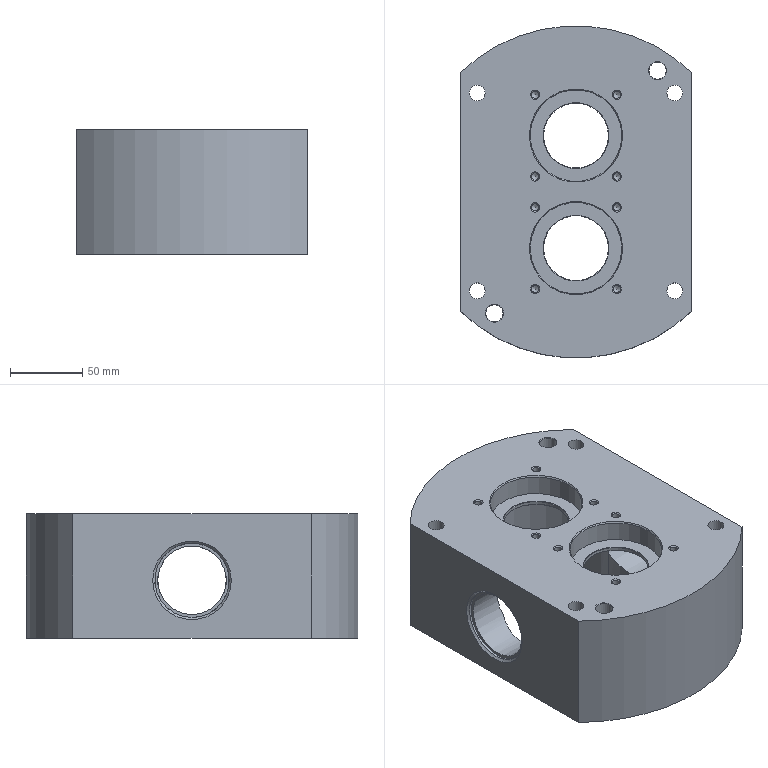NC program | NX | posted with a generic post | part box 160 x 230 x 86 mm
Lines 1 to 2290 of 2342, first 2014 of 2276 lines:
N10 G17 G21 G94 G90
(FLOOR_WALL , TOOL : D50)
N12 T02 M6
N14 G54
N16 G17 G0 G90 X46.956 Y-52.997 B0. C0. S1200 M3
N18 G43 Z30. H2
N20 Z2.651
N22 G94 G1 Z-0.349 F1000.
N24 X43.956
N26 X-43.956 F2000.
N28 Y-24.331
N30 X43.956
N32 Y4.334
N34 X-43.956
N36 Y33.
N38 X43.956
N40 X46.956
N42 Z2.651
N44 G0 Z30.
N46 X50.654 Y-52.997
N48 Z2.302
N50 G1 Z-0.698 F1000.
N52 X47.654
N54 X-47.654 F2000.
N56 Y-24.331
N58 X47.654
N60 Y4.334
N62 X-47.654
N64 Y33.
N66 X47.654
N68 X50.654
N70 Z2.302
N72 G0 Z30.
N74 X53.485 Y-52.997
N76 Z1.953
N78 G1 Z-1.047 F1000.
N80 X50.485
N82 X-50.485 F2000.
N84 Y-24.331
N86 X50.485
N88 Y4.334
N90 X-50.485
N92 Y33.
N94 X50.485
N96 X53.485
N98 Z1.953
N100 G0 Z30.
N102 X55.866 Y-52.997
N104 Z1.604
N106 G1 Z-1.396 F1000.
N108 X52.866
N110 X-52.866 F2000.
N112 Y-24.331
N114 X52.866
N116 Y4.334
N118 X-52.866
N120 Y33.
N122 X52.866
N124 X55.866
N126 Z1.604
N128 G0 Z30.
N130 X57.959 Y-52.997
N132 Z1.255
N134 G1 Z-1.745 F1000.
N136 X54.959
N138 X-54.959 F2000.
N140 Y-24.331
N142 X54.959
N144 Y4.334
N146 X-54.959
N148 Y33.
N150 X54.959
N152 X57.959
N154 Z1.255
N156 G0 Z30.
N158 X59.847 Y-52.997
N160 Z0.906
N162 G1 Z-2.094 F1000.
N164 X56.847
N166 X-56.847 F2000.
N168 Y-24.331
N170 X56.847
N172 Y4.334
N174 X-56.847
N176 Y33.
N178 X56.847
N180 X59.847
N182 Z0.906
N184 G0 Z30.
N186 X61.579 Y-52.997
N188 Z0.557
N190 G1 Z-2.443 F1000.
N192 X58.579
N194 X-58.579 F2000.
N196 Y-24.331
N198 X58.579
N200 Y4.334
N202 X-58.579
N204 Y33.
N206 X58.579
N208 X61.579
N210 Z0.557
N212 G0 Z30.
N214 X63.188 Y-52.997
N216 Z0.208
N218 G1 Z-2.792 F1000.
N220 X60.188
N222 X-60.188 F2000.
N224 Y-24.331
N226 X60.188
N228 Y4.334
N230 X-60.188
N232 Y33.
N234 X60.188
N236 X63.188
N238 Z0.208
N240 G0 Z30.
N242 X64.695 Y-52.997
N244 Z-0.141
N246 G1 Z-3.141 F1000.
N248 X61.695
N250 X-61.695 F2000.
N252 Y-24.331
N254 X61.695
N256 Y4.334
N258 X-61.695
N260 Y33.
N262 X61.695
N264 X64.695
N266 Z-0.141
N268 G0 Z30.
N270 X66.117 Y-52.997
N272 Z-0.49
N274 G1 Z-3.49 F1000.
N276 X63.117
N278 X-63.117 F2000.
N280 Y-24.331
N282 X63.117
N284 Y4.334
N286 X-63.117
N288 Y33.
N290 X63.117
N292 X66.117
N294 Z-0.49
N296 G0 Z30.
N298 X67.467 Y-52.997
N300 Z-0.839
N302 G1 Z-3.839 F1000.
N304 X64.467
N306 X-64.467 F2000.
N308 Y-24.331
N310 X64.467
N312 Y4.334
N314 X-64.467
N316 Y33.
N318 X64.467
N320 X67.467
N322 Z-0.839
N324 G0 Z30.
N326 X68.753 Y-52.997
N328 Z-1.188
N330 G1 Z-4.188 F1000.
N332 X65.753
N334 X-65.753 F2000.
N336 Y-24.331
N338 X65.753
N340 Y4.334
N342 X-65.753
N344 Y33.
N346 X65.753
N348 X68.753
N350 Z-1.188
N352 G0 Z30.
N354 X69.984 Y-52.997
N356 Z-1.537
N358 G1 Z-4.537 F1000.
N360 X66.984
N362 X-66.984 F2000.
N364 Y-24.331
N366 X66.984
N368 Y4.334
N370 X-66.984
N372 Y33.
N374 X66.984
N376 X69.984
N378 Z-1.537
N380 G0 Z30.
N382 X71.166 Y-52.997
N384 Z-1.886
N386 G1 Z-4.886 F1000.
N388 X68.166
N390 X-68.166 F2000.
N392 Y-24.331
N394 X68.166
N396 Y4.334
N398 X-68.166
N400 Y33.
N402 X68.166
N404 X71.166
N406 Z-1.886
N408 G0 Z30.
N410 X72.303 Y-52.997
N412 Z-2.235
N414 G1 Z-5.235 F1000.
N416 X69.303
N418 X-69.303 F2000.
N420 Y-24.331
N422 X69.303
N424 Y4.334
N426 X-69.303
N428 Y33.
N430 X69.303
N432 X72.303
N434 Z-2.235
N436 G0 Z30.
N438 X73.4 Y-52.997
N440 Z-2.584
N442 G1 Z-5.584 F1000.
N444 X70.4
N446 X-70.4 F2000.
N448 Y-24.331
N450 X70.4
N452 Y4.334
N454 X-70.4
N456 Y33.
N458 X70.4
N460 X73.4
N462 Z-2.584
N464 G0 Z30.
N466 X74.462 Y-52.997
N468 Z-2.933
N470 G1 Z-5.933 F1000.
N472 X71.462
N474 X-71.462 F2000.
N476 Y-24.331
N478 X71.462
N480 Y4.334
N482 X-71.462
N484 Y33.
N486 X71.462
N488 X74.462
N490 Z-2.933
N492 G0 Z30.
N494 X75.489 Y-52.997
N496 Z-3.282
N498 G1 Z-6.282 F1000.
N500 X72.489
N502 X-72.489 F2000.
N504 Y-24.331
N506 X72.489
N508 Y4.334
N510 X-72.489
N512 Y33.
N514 X72.489
N516 X75.489
N518 Z-3.282
N520 G0 Z30.
N522 X76.487 Y-52.997
N524 Z-3.631
N526 G1 Z-6.631 F1000.
N528 X73.487
N530 X-73.487 F2000.
N532 Y-24.331
N534 X73.487
N536 Y4.334
N538 X-73.487
N540 Y33.
N542 X73.487
N544 X76.487
N546 Z-3.631
N548 G0 Z30.
N550 X77.455 Y-52.997
N552 Z-3.98
N554 G1 Z-6.98 F1000.
N556 X74.455
N558 X-74.455 F2000.
N560 Y-24.331
N562 X74.455
N564 Y4.334
N566 X-74.455
N568 Y33.
N570 X74.455
N572 X77.455
N574 Z-3.98
N576 G0 Z30.
N578 X78.398 Y-52.997
N580 Z-4.329
N582 G1 Z-7.329 F1000.
N584 X75.398
N586 X-75.398 F2000.
N588 Y-24.331
N590 X75.398
N592 Y4.334
N594 X-75.398
N596 Y33.
N598 X75.398
N600 X78.398
N602 Z-4.329
N604 G0 Z30.
N606 X79.316 Y-52.997
N608 Z-4.678
N610 G1 Z-7.678 F1000.
N612 X76.316
N614 X-76.316 F2000.
N616 Y-24.331
N618 X76.316
N620 Y4.334
N622 X-76.316
N624 Y33.
N626 X76.316
N628 X79.316
N630 Z-4.678
N632 G0 Z30.
N634 X80.212 Y-52.997
N636 Z-5.027
N638 G1 Z-8.027 F1000.
N640 X77.212
N642 X-77.212 F2000.
N644 Y-24.331
N646 X77.212
N648 Y4.334
N650 X-77.212
N652 Y33.
N654 X77.212
N656 X80.212
N658 Z-5.027
N660 G0 Z30.
N662 X81.086 Y-52.997
N664 Z-5.376
N666 G1 Z-8.376 F1000.
N668 X78.086
N670 X-78.086 F2000.
N672 Y-24.331
N674 X78.086
N676 Y4.334
N678 X-78.086
N680 Y33.
N682 X78.086
N684 X81.086
N686 Z-5.376
N688 G0 Z30.
N690 X81.939 Y-52.997
N692 Z-5.725
N694 G1 Z-8.725 F1000.
N696 X78.939
N698 X-78.939 F2000.
N700 Y-24.331
N702 X78.939
N704 Y4.334
N706 X-78.939
N708 Y33.
N710 X78.939
N712 X81.939
N714 Z-5.725
N716 G0 Z30.
N718 X82.774 Y-52.997
N720 Z-6.074
N722 G1 Z-9.074 F1000.
N724 X79.774
N726 X-79.774 F2000.
N728 Y-24.331
N730 X79.774
N732 Y4.334
N734 X-79.774
N736 Y33.
N738 X79.774
N740 X82.774
N742 Z-6.074
N744 G0 Z30.
N746 X83.591 Y-52.997
N748 Z-6.423
N750 G1 Z-9.423 F1000.
N752 X80.591
N754 X-80.591 F2000.
N756 Y-24.331
N758 X80.591
N760 Y4.334
N762 X-80.591
N764 Y33.
N766 X80.591
N768 X83.591
N770 Z-6.423
N772 G0 Z30.
N774 X84.391 Y-52.997
N776 Z-6.772
N778 G1 Z-9.772 F1000.
N780 X81.391
N782 X-81.391 F2000.
N784 Y-24.331
N786 X81.391
N788 Y4.334
N790 X-81.391
N792 Y33.
N794 X81.391
N796 X84.391
N798 Z-6.772
N800 G0 Z30.
N802 X85.175 Y-52.997
N804 Z-7.121
N806 G1 Z-10.121 F1000.
N808 X82.175
N810 X-82.175 F2000.
N812 Y-24.331
N814 X82.175
N816 Y4.334
N818 X-82.175
N820 Y33.
N822 X82.175
N824 X85.175
N826 Z-7.121
N828 G0 Z30.
N830 X85.943 Y-52.997
N832 Z-7.47
N834 G1 Z-10.47 F1000.
N836 X82.943
N838 X-82.943 F2000.
N840 Y-24.331
N842 X82.943
N844 Y4.334
N846 X-82.943
N848 Y33.
N850 X82.943
N852 X85.943
N854 Z-7.47
N856 G0 Z30.
N858 X86.697 Y-52.997
N860 Z-7.819
N862 G1 Z-10.819 F1000.
N864 X83.697
N866 X-83.697 F2000.
N868 Y-24.331
N870 X83.697
N872 Y4.334
N874 X-83.697
N876 Y33.
N878 X83.697
N880 X86.697
N882 Z-7.819
N884 G0 Z30.
N886 X87.436 Y-52.997
N888 Z-8.168
N890 G1 Z-11.168 F1000.
N892 X84.436
N894 X-84.436 F2000.
N896 Y-24.331
N898 X84.436
N900 Y4.334
N902 X-84.436
N904 Y33.
N906 X84.436
N908 X87.436
N910 Z-8.168
N912 G0 Z30.
N914 X88.163 Y-52.997
N916 Z-8.517
N918 G1 Z-11.517 F1000.
N920 X85.163
N922 X-85.163 F2000.
N924 Y-24.331
N926 X85.163
N928 Y4.334
N930 X-85.163
N932 Y33.
N934 X85.163
N936 X88.163
N938 Z-8.517
N940 G0 Z30.
N942 X88.877 Y-52.997
N944 Z-8.866
N946 G1 Z-11.866 F1000.
N948 X85.877
N950 X-85.877 F2000.
N952 Y-24.331
N954 X85.877
N956 Y4.334
N958 X-85.877
N960 Y33.
N962 X85.877
N964 X88.877
N966 Z-8.866
N968 G0 Z30.
N970 X89.578 Y-52.997
N972 Z-9.215
N974 G1 Z-12.215 F1000.
N976 X86.578
N978 X-86.578 F2000.
N980 Y-24.331
N982 X86.578
N984 Y4.334
N986 X-86.578
N988 Y33.
N990 X86.578
N992 X89.578
N994 Z-9.215
N996 G0 Z30.
N998 X90.268 Y-52.997
N1000 Z-9.564
N1002 G1 Z-12.564 F1000.
N1004 X87.268
N1006 X-87.268 F2000.
N1008 Y-24.331
N1010 X87.268
N1012 Y4.334
N1014 X-87.268
N1016 Y33.
N1018 X87.268
N1020 X90.268
N1022 Z-9.564
N1024 G0 Z30.
N1026 X90.946 Y-52.997
N1028 Z-9.913
N1030 G1 Z-12.913 F1000.
N1032 X87.946
N1034 X-87.946 F2000.
N1036 Y-24.331
N1038 X87.946
N1040 Y4.334
N1042 X-87.946
N1044 Y33.
N1046 X87.946
N1048 X90.946
N1050 Z-9.913
N1052 G0 Z30.
N1054 X91.614 Y-52.997
N1056 Z-10.262
N1058 G1 Z-13.262 F1000.
N1060 X88.614
N1062 X-88.614 F2000.
N1064 Y-24.331
N1066 X88.614
N1068 Y4.334
N1070 X-88.614
N1072 Y33.
N1074 X88.614
N1076 X91.614
N1078 Z-10.262
N1080 G0 Z30.
N1082 X92.271 Y-52.997
N1084 Z-10.611
N1086 G1 Z-13.611 F1000.
N1088 X89.271
N1090 X-89.271 F2000.
N1092 Y-24.331
N1094 X89.271
N1096 Y4.334
N1098 X-89.271
N1100 Y33.
N1102 X89.271
N1104 X92.271
N1106 Z-10.611
N1108 G0 Z30.
N1110 X92.918 Y-52.997
N1112 Z-10.96
N1114 G1 Z-13.96 F1000.
N1116 X89.918
N1118 X-89.918 F2000.
N1120 Y-24.331
N1122 X89.918
N1124 Y4.334
N1126 X-89.918
N1128 Y33.
N1130 X89.918
N1132 X92.918
N1134 Z-10.96
N1136 G0 Z30.
N1138 X93.555 Y-52.997
N1140 Z-11.309
N1142 G1 Z-14.309 F1000.
N1144 X90.555
N1146 X-90.555 F2000.
N1148 Y-24.331
N1150 X90.555
N1152 Y4.334
N1154 X-90.555
N1156 Y33.
N1158 X90.555
N1160 X93.555
N1162 Z-11.309
N1164 G0 Z30.
N1166 X94.183 Y-52.997
N1168 Z-11.658
N1170 G1 Z-14.658 F1000.
N1172 X91.183
N1174 X-91.183 F2000.
N1176 Y-24.331
N1178 X91.183
N1180 Y4.334
N1182 X-91.183
N1184 Y33.
N1186 X91.183
N1188 X94.183
N1190 Z-11.658
N1192 G0 Z30.
N1194 X94.802 Y-52.997
N1196 Z-12.007
N1198 G1 Z-15.007 F1000.
N1200 X91.802
N1202 X-91.802 F2000.
N1204 Y-24.331
N1206 X91.802
N1208 Y4.334
N1210 X-91.802
N1212 Y33.
N1214 X91.802
N1216 X94.802
N1218 Z-12.007
N1220 G0 Z30.
N1222 X95.412 Y-52.997
N1224 Z-12.356
N1226 G1 Z-15.356 F1000.
N1228 X92.412
N1230 X-92.412 F2000.
N1232 Y-24.331
N1234 X92.412
N1236 Y4.334
N1238 X-92.412
N1240 Y33.
N1242 X92.412
N1244 X95.412
N1246 Z-12.356
N1248 G0 Z30.
N1250 X96.013 Y-52.997
N1252 Z-12.705
N1254 G1 Z-15.705 F1000.
N1256 X93.013
N1258 X-93.013 F2000.
N1260 Y-24.331
N1262 X93.013
N1264 Y4.334
N1266 X-93.013
N1268 Y33.
N1270 X93.013
N1272 X96.013
N1274 Z-12.705
N1276 G0 Z30.
N1278 X96.606 Y-52.997
N1280 Z-13.054
N1282 G1 Z-16.054 F1000.
N1284 X93.606
N1286 X-93.606 F2000.
N1288 Y-24.331
N1290 X93.606
N1292 Y4.334
N1294 X-93.606
N1296 Y33.
N1298 X93.606
N1300 X96.606
N1302 Z-13.054
N1304 G0 Z30.
N1306 X97.192 Y-52.997
N1308 Z-13.403
N1310 G1 Z-16.403 F1000.
N1312 X94.192
N1314 X-94.192 F2000.
N1316 Y-24.331
N1318 X94.192
N1320 Y4.334
N1322 X-94.192
N1324 Y33.
N1326 X94.192
N1328 X97.192
N1330 Z-13.403
N1332 G0 Z30.
N1334 X97.769 Y-52.997
N1336 Z-13.752
N1338 G1 Z-16.752 F1000.
N1340 X94.769
N1342 X-94.769 F2000.
N1344 Y-24.331
N1346 X94.769
N1348 Y4.334
N1350 X-94.769
N1352 Y33.
N1354 X94.769
N1356 X97.769
N1358 Z-13.752
N1360 G0 Z30.
N1362 X98.339 Y-52.997
N1364 Z-14.101
N1366 G1 Z-17.101 F1000.
N1368 X95.339
N1370 X-95.339 F2000.
N1372 Y-24.331
N1374 X95.339
N1376 Y4.334
N1378 X-95.339
N1380 Y33.
N1382 X95.339
N1384 X98.339
N1386 Z-14.101
N1388 G0 Z30.
N1390 X98.902 Y-52.997
N1392 Z-14.45
N1394 G1 Z-17.45 F1000.
N1396 X95.902
N1398 X-95.902 F2000.
N1400 Y-24.331
N1402 X95.902
N1404 Y4.334
N1406 X-95.902
N1408 Y33.
N1410 X95.902
N1412 X98.902
N1414 Z-14.45
N1416 G0 Z30.
N1418 X99.457 Y-52.997
N1420 Z-14.799
N1422 G1 Z-17.799 F1000.
N1424 X96.457
N1426 X-96.457 F2000.
N1428 Y-24.331
N1430 X96.457
N1432 Y4.334
N1434 X-96.457
N1436 Y33.
N1438 X96.457
N1440 X99.457
N1442 Z-14.799
N1444 G0 Z30.
N1446 X100.006 Y-52.997
N1448 Z-15.148
N1450 G1 Z-18.148 F1000.
N1452 X97.006
N1454 X-97.006 F2000.
N1456 Y-24.331
N1458 X97.006
N1460 Y4.334
N1462 X-97.006
N1464 Y33.
N1466 X97.006
N1468 X100.006
N1470 Z-15.148
N1472 G0 Z30.
N1474 X100.548 Y-52.997
N1476 Z-15.497
N1478 G1 Z-18.497 F1000.
N1480 X97.548
N1482 X-97.548 F2000.
N1484 Y-24.331
N1486 X97.548
N1488 Y4.334
N1490 X-97.548
N1492 Y33.
N1494 X97.548
N1496 X100.548
N1498 Z-15.497
N1500 G0 Z30.
N1502 X101.083 Y-52.997
N1504 Z-15.846
N1506 G1 Z-18.846 F1000.
N1508 X98.083
N1510 X-98.083 F2000.
N1512 Y-24.331
N1514 X98.083
N1516 Y4.334
N1518 X-98.083
N1520 Y33.
N1522 X98.083
N1524 X101.083
N1526 Z-15.846
N1528 G0 Z30.
N1530 X101.612 Y-52.997
N1532 Z-16.195
N1534 G1 Z-19.195 F1000.
N1536 X98.612
N1538 X-98.612 F2000.
N1540 Y-24.331
N1542 X98.612
N1544 Y4.334
N1546 X-98.612
N1548 Y33.
N1550 X98.612
N1552 X101.612
N1554 Z-16.195
N1556 G0 Z30.
N1558 X102.134 Y-52.997
N1560 Z-16.544
N1562 G1 Z-19.544 F1000.
N1564 X99.134
N1566 X-99.134 F2000.
N1568 Y-24.331
N1570 X99.134
N1572 Y4.334
N1574 X-99.134
N1576 Y33.
N1578 X99.134
N1580 X102.134
N1582 Z-16.544
N1584 G0 Z30.
N1586 X102.65 Y-52.997
N1588 Z-16.893
N1590 G1 Z-19.893 F1000.
N1592 X99.65
N1594 X-99.65 F2000.
N1596 Y-24.331
N1598 X99.65
N1600 Y4.334
N1602 X-99.65
N1604 Y33.
N1606 X99.65
N1608 X102.65
N1610 Z-16.893
N1612 G0 Z30.
N1614 X103.161 Y-52.997
N1616 Z-17.242
N1618 G1 Z-20.242 F1000.
N1620 X100.161
N1622 X-100.161 F2000.
N1624 Y-24.331
N1626 X100.161
N1628 Y4.334
N1630 X-100.161
N1632 Y33.
N1634 X100.161
N1636 X103.161
N1638 Z-17.242
N1640 G0 Z30.
N1642 X103.666 Y-52.997
N1644 Z-17.591
N1646 G1 Z-20.591 F1000.
N1648 X100.666
N1650 X-100.666 F2000.
N1652 Y-24.331
N1654 X100.666
N1656 Y4.334
N1658 X-100.666
N1660 Y33.
N1662 X100.666
N1664 X103.666
N1666 Z-17.591
N1668 G0 Z30.
N1670 X104.164 Y-52.997
N1672 Z-17.94
N1674 G1 Z-20.94 F1000.
N1676 X101.164
N1678 X-101.164 F2000.
N1680 Y-24.331
N1682 X101.164
N1684 Y4.334
N1686 X-101.164
N1688 Y33.
N1690 X101.164
N1692 X104.164
N1694 Z-17.94
N1696 G0 Z30.
N1698 X104.658 Y-52.997
N1700 Z-18.289
N1702 G1 Z-21.289 F1000.
N1704 X101.658
N1706 X-101.658 F2000.
N1708 Y-24.331
N1710 X101.658
N1712 Y4.334
N1714 X-101.658
N1716 Y33.
N1718 X101.658
N1720 X104.658
N1722 Z-18.289
N1724 G0 Z30.
N1726 X105.146 Y-52.997
N1728 Z-18.638
N1730 G1 Z-21.638 F1000.
N1732 X102.146
N1734 X-102.146 F2000.
N1736 Y-24.331
N1738 X102.146
N1740 Y4.334
N1742 X-102.146
N1744 Y33.
N1746 X102.146
N1748 X105.146
N1750 Z-18.638
N1752 G0 Z30.
N1754 X105.628 Y-52.997
N1756 Z-18.987
N1758 G1 Z-21.987 F1000.
N1760 X102.628
N1762 X-102.628 F2000.
N1764 Y-24.331
N1766 X102.628
N1768 Y4.334
N1770 X-102.628
N1772 Y33.
N1774 X102.628
N1776 X105.628
N1778 Z-18.987
N1780 G0 Z30.
N1782 X106.106 Y-52.997
N1784 Z-19.336
N1786 G1 Z-22.336 F1000.
N1788 X103.106
N1790 X-103.106 F2000.
N1792 Y-24.331
N1794 X103.106
N1796 Y4.334
N1798 X-103.106
N1800 Y33.
N1802 X103.106
N1804 X106.106
N1806 Z-19.336
N1808 G0 Z30.
N1810 X106.578 Y-52.997
N1812 Z-19.685
N1814 G1 Z-22.685 F1000.
N1816 X103.578
N1818 X-103.578 F2000.
N1820 Y-24.331
N1822 X103.578
N1824 Y4.334
N1826 X-103.578
N1828 Y33.
N1830 X103.578
N1832 X106.578
N1834 Z-19.685
N1836 G0 Z30.
N1838 X107.045 Y-52.997
N1840 Z-20.034
N1842 G1 Z-23.034 F1000.
N1844 X104.045
N1846 X-104.045 F2000.
N1848 Y-24.331
N1850 X104.045
N1852 Y4.334
N1854 X-104.045
N1856 Y33.
N1858 X104.045
N1860 X107.045
N1862 Z-20.034
N1864 G0 Z30.
N1866 X107.508 Y-52.997
N1868 Z-20.383
N1870 G1 Z-23.383 F1000.
N1872 X104.508
N1874 X-104.508 F2000.
N1876 Y-24.331
N1878 X104.508
N1880 Y4.334
N1882 X-104.508
N1884 Y33.
N1886 X104.508
N1888 X107.508
N1890 Z-20.383
N1892 G0 Z30.
N1894 X107.965 Y-52.997
N1896 Z-20.732
N1898 G1 Z-23.732 F1000.
N1900 X104.965
N1902 X-104.965 F2000.
N1904 Y-24.331
N1906 X104.965
N1908 Y4.334
N1910 X-104.965
N1912 Y33.
N1914 X104.965
N1916 X107.965
N1918 Z-20.732
N1920 G0 Z30.
N1922 X108.418 Y-52.997
N1924 Z-21.081
N1926 G1 Z-24.081 F1000.
N1928 X105.418
N1930 X-105.418 F2000.
N1932 Y-24.331
N1934 X105.418
N1936 Y4.334
N1938 X-105.418
N1940 Y33.
N1942 X105.418
N1944 X108.418
N1946 Z-21.081
N1948 G0 Z30.
N1950 X108.867 Y-52.997
N1952 Z-21.43
N1954 G1 Z-24.43 F1000.
N1956 X105.867
N1958 X-105.867 F2000.
N1960 Y-24.331
N1962 X105.867
N1964 Y4.334
N1966 X-105.867
N1968 Y33.
N1970 X105.867
N1972 X108.867
N1974 Z-21.43
N1976 G0 Z30.
N1978 X109.31 Y-52.997
N1980 Z-21.779
N1982 G1 Z-24.779 F1000.
N1984 X106.31
N1986 X-106.31 F2000.
N1988 Y-24.331
N1990 X106.31
N1992 Y4.334
N1994 X-106.31
N1996 Y33.
N1998 X106.31
N2000 X109.31
N2002 Z-21.779
N2004 G0 Z30.
N2006 X109.75 Y-52.997
N2008 Z-22.128
N2010 G1 Z-25.128 F1000.
N2012 X106.75
N2014 X-106.75 F2000.
N2016 Y-24.331
N2018 X106.75
N2020 Y4.334
N2022 X-106.75
N2024 Y33.
N2026 X106.75
N2028 X109.75
N2030 Z-22.128
N2032 G0 Z30.
N2034 X110.185 Y-52.997
N2036 Z-22.477
N2038 G1 Z-25.477 F1000.
N2040 X107.185
N2042 X-107.185 F2000.
N2044 Y-24.331
N2046 X107.185
N2048 Y4.334
N2050 X-107.185
N2052 Y33.
N2054 X107.185
N2056 X110.185
N2058 Z-22.477
N2060 G0 Z30.
N2062 X110.616 Y-52.997
N2064 Z-22.826
N2066 G1 Z-25.826 F1000.
N2068 X107.616
N2070 X-107.616 F2000.
N2072 Y-24.331
N2074 X107.616
N2076 Y4.334
N2078 X-107.616
N2080 Y33.
N2082 X107.616
N2084 X110.616
N2086 Z-22.826
N2088 G0 Z30.
N2090 X111.042 Y-52.997
N2092 Z-23.175
N2094 G1 Z-26.175 F1000.
N2096 X108.042
N2098 X-108.042 F2000.
N2100 Y-24.331
N2102 X108.042
N2104 Y4.334
N2106 X-108.042
N2108 Y33.
N2110 X108.042
N2112 X111.042
N2114 Z-23.175
N2116 G0 Z30.
N2118 X111.464 Y-52.997
N2120 Z-23.524
N2122 G1 Z-26.524 F1000.
N2124 X108.464
N2126 X-108.464 F2000.
N2128 Y-24.331
N2130 X108.464
N2132 Y4.334
N2134 X-108.464
N2136 Y33.
N2138 X108.464
N2140 X111.464
N2142 Z-23.524
N2144 G0 Z30.
N2146 X111.883 Y-52.997
N2148 Z-23.873
N2150 G1 Z-26.873 F1000.
N2152 X108.883
N2154 X-108.883 F2000.
N2156 Y-24.331
N2158 X108.883
N2160 Y4.334
N2162 X-108.883
N2164 Y33.
N2166 X108.883
N2168 X111.883
N2170 Z-23.873
N2172 G0 Z30.
N2174 X112.297 Y-52.997
N2176 Z-24.222
N2178 G1 Z-27.222 F1000.
N2180 X109.297
N2182 X-109.297 F2000.
N2184 Y-24.331
N2186 X109.297
N2188 Y4.334
N2190 X-109.297
N2192 Y33.
N2194 X109.297
N2196 X112.297
N2198 Z-24.222
N2200 G0 Z30.
N2202 X112.707 Y-52.997
N2204 Z-24.571
N2206 G1 Z-27.571 F1000.
N2208 X109.707
N2210 X-109.707 F2000.
N2212 Y-24.331
N2214 X109.707
N2216 Y4.334
N2218 X-109.707
N2220 Y33.
N2222 X109.707
N2224 X112.707
N2226 Z-24.571
N2228 G0 Z30.
N2230 X113.114 Y-52.997
N2232 Z-24.92
N2234 G1 Z-27.92 F1000.
N2236 X110.114
N2238 X-110.114 F2000.
N2240 Y-24.331
N2242 X110.114
N2244 Y4.334
N2246 X-110.114
N2248 Y33.
N2250 X110.114
N2252 X113.114
N2254 Z-24.92
N2256 G0 Z30.
N2258 X113.517 Y-52.997
N2260 Z-25.269
N2262 G1 Z-28.269 F1000.
N2264 X110.517
N2266 X-110.517 F2000.
N2268 Y-24.331
N2270 X110.517
N2272 Y4.334
N2274 X-110.517
N2276 Y33.
N2278 X110.517
N2280 X113.517
N2282 Z-25.269
N2284 G0 Z30.
N2286 X113.915 Y-52.997
N2288 Z-25.618
N2290 G1 Z-28.618 F1000.
N2292 X110.915
N2294 X-110.915 F2000.
N2296 Y-24.331
N2298 X110.915
N2300 Y4.334
N2302 X-110.915
N2304 Y33.
N2306 X110.915
N2308 X113.915
N2310 Z-25.618
N2312 G0 Z30.
N2314 X114.311 Y-52.997
N2316 Z-25.967
N2318 G1 Z-28.967 F1000.
N2320 X111.311
N2322 X-111.311 F2000.
N2324 Y-24.331
N2326 X111.311
N2328 Y4.334
N2330 X-111.311
N2332 Y33.
N2334 X111.311
N2336 X114.311
N2338 Z-25.967
N2340 G0 Z30.
N2342 X114.702 Y-52.997
N2344 Z-26.316
N2346 G1 Z-29.316 F1000.
N2348 X111.702
N2350 X-111.702 F2000.
N2352 Y-24.331
N2354 X111.702
N2356 Y4.334
N2358 X-111.702
N2360 Y33.
N2362 X111.702
N2364 X114.702
N2366 Z-26.316
N2368 G0 Z30.
N2370 X115.091 Y-52.997
N2372 Z-26.665
N2374 G1 Z-29.665 F1000.
N2376 X112.091
N2378 X-112.091 F2000.
N2380 Y-24.331
N2382 X112.091
N2384 Y4.334
N2386 X-112.091
N2388 Y33.
N2390 X112.091
N2392 X115.091
N2394 Z-26.665
N2396 G0 Z30.
N2398 X115.475 Y-52.997
N2400 Z-27.014
N2402 G1 Z-30.014 F1000.
N2404 X112.475
N2406 X-112.475 F2000.
N2408 Y-24.331
N2410 X112.475
N2412 Y4.334
N2414 X-112.475
N2416 Y33.
N2418 X112.475
N2420 X115.475
N2422 Z-27.014
N2424 G0 Z30.
N2426 X115.856 Y-52.997
N2428 Z-27.363
N2430 G1 Z-30.363 F1000.
N2432 X112.856
N2434 X-112.856 F2000.
N2436 Y-24.331
N2438 X112.856
N2440 Y4.334
N2442 X-112.856
N2444 Y33.
N2446 X112.856
N2448 X115.856
N2450 Z-27.363
N2452 G0 Z30.
N2454 X116.234 Y-52.997
N2456 Z-27.712
N2458 G1 Z-30.712 F1000.
N2460 X113.234
N2462 X-113.234 F2000.
N2464 Y-24.331
N2466 X113.234
N2468 Y4.334
N2470 X-113.234
N2472 Y33.
N2474 X113.234
N2476 X116.234
N2478 Z-27.712
N2480 G0 Z30.
N2482 X116.608 Y-52.997
N2484 Z-28.061
N2486 G1 Z-31.061 F1000.
N2488 X113.608
N2490 X-113.608 F2000.
N2492 Y-24.331
N2494 X113.608
N2496 Y4.334
N2498 X-113.608
N2500 Y33.
N2502 X113.608
N2504 X116.608
N2506 Z-28.061
N2508 G0 Z30.
N2510 X116.979 Y-52.997
N2512 Z-28.41
N2514 G1 Z-31.41 F1000.
N2516 X113.979
N2518 X-113.979 F2000.
N2520 Y-24.331
N2522 X113.979
N2524 Y4.334
N2526 X-113.979
N2528 Y33.
N2530 X113.979
N2532 X116.979
N2534 Z-28.41
N2536 G0 Z30.
N2538 X117.347 Y-52.997
N2540 Z-28.759
N2542 G1 Z-31.759 F1000.
N2544 X114.347
N2546 X-114.347 F2000.
N2548 Y-24.331
N2550 X114.347
N2552 Y4.334
N2554 X-114.347
N2556 Y33.
N2558 X114.347
N2560 X117.347
N2562 Z-28.759
N2564 G0 Z30.
N2566 X117.711 Y-52.997
N2568 Z-29.108
N2570 G1 Z-32.108 F1000.
N2572 X114.711
N2574 X-114.711 F2000.
N2576 Y-24.331
N2578 X114.711
N2580 Y4.334
N2582 X-114.711
N2584 Y33.
N2586 X114.711
N2588 X117.711
N2590 Z-29.108
N2592 G0 Z30.
N2594 X118.073 Y-52.997
N2596 Z-29.457
N2598 G1 Z-32.457 F1000.
N2600 X115.073
N2602 X-115.073 F2000.
N2604 Y-24.331
N2606 X115.073
N2608 Y4.334
N2610 X-115.073
N2612 Y33.
N2614 X115.073
N2616 X118.073
N2618 Z-29.457
N2620 G0 Z30.
N2622 X118.431 Y-52.997
N2624 Z-29.806
N2626 G1 Z-32.806 F1000.
N2628 X115.431
N2630 X-115.431 F2000.
N2632 Y-24.331
N2634 X115.431
N2636 Y4.334
N2638 X-115.431
N2640 Y33.
N2642 X115.431
N2644 X118.431
N2646 Z-29.806
N2648 G0 Z30.
N2650 X118.786 Y-52.997
N2652 Z-30.155
N2654 G1 Z-33.155 F1000.
N2656 X115.786
N2658 X-115.786 F2000.
N2660 Y-24.331
N2662 X115.786
N2664 Y4.334
N2666 X-115.786
N2668 Y33.
N2670 X115.786
N2672 X118.786
N2674 Z-30.155
N2676 G0 Z30.
N2678 X119.138 Y-52.997
N2680 Z-30.504
N2682 G1 Z-33.504 F1000.
N2684 X116.138
N2686 X-116.138 F2000.
N2688 Y-24.331
N2690 X116.138
N2692 Y4.334
N2694 X-116.138
N2696 Y33.
N2698 X116.138
N2700 X119.138
N2702 Z-30.504
N2704 G0 Z30.
N2706 X119.487 Y-52.997
N2708 Z-30.853
N2710 G1 Z-33.853 F1000.
N2712 X116.487
N2714 X-116.487 F2000.
N2716 Y-24.331
N2718 X116.487
N2720 Y4.334
N2722 X-116.487
N2724 Y33.
N2726 X116.487
N2728 X119.487
N2730 Z-30.853
N2732 G0 Z30.
N2734 X119.833 Y-52.997
N2736 Z-31.202
N2738 G1 Z-34.202 F1000.
N2740 X116.833
N2742 X-116.833 F2000.
N2744 Y-24.331
N2746 X116.833
N2748 Y4.334
N2750 X-116.833
N2752 Y33.
N2754 X116.833
N2756 X119.833
N2758 Z-31.202
N2760 G0 Z30.
N2762 X120.176 Y-52.997
N2764 Z-31.551
N2766 G1 Z-34.551 F1000.
N2768 X117.176
N2770 X-117.176 F2000.
N2772 Y-24.331
N2774 X117.176
N2776 Y4.334
N2778 X-117.176
N2780 Y33.
N2782 X117.176
N2784 X120.176
N2786 Z-31.551
N2788 G0 Z30.
N2790 X120.517 Y-52.997
N2792 Z-31.9
N2794 G1 Z-34.9 F1000.
N2796 X117.517
N2798 X-117.517 F2000.
N2800 Y-24.331
N2802 X117.517
N2804 Y4.334
N2806 X-117.517
N2808 Y33.
N2810 X117.517
N2812 X120.517
N2814 Z-31.9
N2816 G0 Z30.
(FLOOR_WALL_COPY , TOOL : D50)
N2818 X120.614 Y-52.997 S2500
N2820 Z-32.
N2822 G1 Z-35. F1000.
N2824 X117.614
N2826 X-117.614
N2828 Y-24.331
N2830 X117.614
N2832 Y4.334
N2834 X-117.614
N2836 Y33.
N2838 X117.614
N2840 X120.614
N2842 Z-32.
N2844 G0 Z30.
N2846 M5
(HOLE_MILLING , TOOL : D10)
N2848 T10 M6
N2850 G54
N2852 G17 G0 G90 X0. Y-3. B0. C0. S3000 M3
N2854 G43 Z30. H10
N2856 Z-34.5
N2858 G94 G3 X-1.25 Y-1.75 R1.25 F2200.
N2860 X-2.5 Y-3. R1.25
N2862 X-2.5 Y-3. Z-34.72 I2.5 J0.
N2864 X-2.5 Y-3. Z-34.94 I2.5 J0.
N2866 X-2.5 Y-3. Z-35.16 I2.5 J0.
N2868 X-2.5 Y-3. Z-35.38 I2.5 J0.
N2870 X-2.5 Y-3. Z-35.6 I2.5 J0.
N2872 X-2.5 Y-3. Z-35.82 I2.5 J0.
N2874 X-2.5 Y-3. Z-36.04 I2.5 J0.
N2876 X-2.5 Y-3. Z-36.26 I2.5 J0.
N2878 X-2.5 Y-3. Z-36.48 I2.5 J0.
N2880 X-2.5 Y-3. Z-36.7 I2.5 J0.
N2882 X-2.5 Y-3. Z-36.92 I2.5 J0.
N2884 X-2.5 Y-3. Z-37.14 I2.5 J0.
N2886 X-2.5 Y-3. Z-37.36 I2.5 J0.
N2888 X-2.5 Y-3. Z-37.58 I2.5 J0.
N2890 X-2.5 Y-3. Z-37.8 I2.5 J0.
N2892 X-2.103 Y-1.648 Z-38. R-2.5
N2894 X-1.34 Y-5.155 R2.538
N2896 X2.196 Y-4.411 R2.572
N2898 X1.453 Y-0.766 R2.63
N2900 X-2.288 Y-1.529 R2.7
N2902 X-1.513 Y-5.326 R2.74
N2904 X2.381 Y-4.53 R2.81
N2906 X1.572 Y-0.581 R2.85
N2908 X-2.473 Y-1.411 R2.92
N2910 X-1.632 Y-5.511 R2.96
N2912 X2.566 Y-4.649 R3.03
N2914 X1.691 Y-0.396 R3.07
N2916 X-2.658 Y-1.292 R3.14
N2918 X-1.751 Y-5.696 R3.18
N2920 X2.751 Y-4.768 R3.25
N2922 X1.81 Y-0.211 R3.29
N2924 X-2.843 Y-1.173 R3.36
N2926 X-1.87 Y-5.881 R3.4
N2928 X2.936 Y-4.887 R3.47
N2930 X1.929 Y-0.026 R3.51
N2932 X-3.029 Y-1.054 R3.58
N2934 X-1.989 Y-6.067 R3.62
N2936 X3.121 Y-5.006 R3.69
N2938 X2.048 Y0.159 R3.73
N2940 X-3.214 Y-0.935 R3.8
N2942 X-2.108 Y-6.252 R3.84
N2944 X3.306 Y-5.125 R3.91
N2946 X2.167 Y0.344 R3.95
N2948 X-3.399 Y-0.816 R4.02
N2950 X-2.227 Y-6.437 R4.06
N2952 X3.491 Y-5.244 R4.13
N2954 X2.286 Y0.529 R4.17
N2956 X-3.584 Y-0.697 R4.24
N2958 X-2.345 Y-6.622 R4.28
N2960 X3.676 Y-5.363 R4.35
N2962 X2.405 Y0.714 R4.39
N2964 X-3.769 Y-0.578 R4.46
N2966 X-2.464 Y-6.807 R4.5
N2968 X3.861 Y-5.482 R4.57
N2970 X2.524 Y0.899 R4.61
N2972 X-3.954 Y-0.459 R4.68
N2974 X-2.583 Y-6.992 R4.72
N2976 X4.046 Y-5.6 R4.79
N2978 X2.643 Y1.084 R4.83
N2980 X-4.139 Y-0.34 R4.9
N2982 X-2.702 Y-7.177 R4.94
N2984 X4.232 Y-5.719 R5.01
N2986 X2.762 Y1.27 R5.05
N2988 X-4.324 Y-0.221 R5.12
N2990 X-2.821 Y-7.362 R5.16
N2992 X4.417 Y-5.838 R5.23
N2994 X2.881 Y1.455 R5.27
N2996 X-4.509 Y-0.102 R5.34
N2998 X-2.94 Y-7.547 R5.38
N3000 X4.602 Y-5.957 R5.45
N3002 X3. Y1.64 R5.49
N3004 X-4.694 Y0.017 R5.56
N3006 X-3.059 Y-7.732 R5.6
N3008 X4.787 Y-6.076 R5.67
N3010 X3.119 Y1.825 R5.71
N3012 X-4.879 Y0.136 R5.78
N3014 X-3.178 Y-7.917 R5.82
N3016 X4.972 Y-6.195 R5.89
N3018 X3.238 Y2.01 R5.93
N3020 X-5.064 Y0.255 R6.
N3022 X-3.297 Y-8.102 R6.04
N3024 X5.157 Y-6.314 R6.11
N3026 X3.356 Y2.195 R6.15
N3028 X-5.249 Y0.374 R6.22
N3030 X-3.416 Y-8.287 R6.26
N3032 X5.342 Y-6.433 R6.33
N3034 X3.475 Y2.38 R6.37
N3036 X-5.434 Y0.493 R6.44
N3038 X-3.535 Y-8.473 R6.48
N3040 X5.527 Y-6.552 R6.55
N3042 X3.594 Y2.565 R6.59
N3044 X-5.62 Y0.611 R6.66
N3046 X-3.654 Y-8.658 R6.7
N3048 X5.712 Y-6.671 R6.77
N3050 X3.713 Y2.75 R6.81
N3052 X-5.805 Y0.73 R6.88
N3054 X-3.773 Y-8.843 R6.92
N3056 X5.897 Y-6.79 R6.99
N3058 X3.832 Y2.935 R7.03
N3060 X-5.99 Y0.849 R7.1
N3062 X-3.892 Y-9.028 R7.14
N3064 X6.082 Y-6.909 R7.21
N3066 X3.951 Y3.12 R7.25
N3068 X-6.175 Y0.968 R7.32
N3070 X-4.011 Y-9.213 R7.36
N3072 X6.267 Y-7.028 R7.43
N3074 X4.07 Y3.305 R7.47
N3076 X-6.36 Y1.087 R7.54
N3078 X-4.13 Y-9.398 R7.58
N3080 X6.452 Y-7.147 R7.65
N3082 X4.189 Y3.491 R7.69
N3084 X-6.545 Y1.206 R7.76
N3086 X-4.249 Y-9.583 R7.8
N3088 X6.637 Y-7.266 R7.87
N3090 X4.308 Y3.676 R7.91
N3092 X-6.73 Y1.325 R7.98
N3094 X-4.367 Y-9.768 R8.02
N3096 X6.823 Y-7.385 R8.09
N3098 X4.427 Y3.861 R8.13
N3100 X-6.915 Y1.444 R8.2
N3102 X-4.486 Y-9.953 R8.24
N3104 X7.008 Y-7.504 R8.31
N3106 X4.546 Y4.046 R8.35
N3108 X-7.1 Y1.563 R8.42
N3110 X-4.605 Y-10.138 R8.46
N3112 X7.193 Y-7.622 R8.53
N3114 X4.665 Y4.231 R8.57
N3116 X-7.285 Y1.682 R8.64
N3118 X-4.724 Y-10.323 R8.68
N3120 X7.378 Y-7.741 R8.75
N3122 X4.784 Y4.416 R8.79
N3124 X-7.47 Y1.801 R8.86
N3126 X-4.843 Y-10.508 R8.9
N3128 X7.563 Y-7.86 R8.97
N3130 X4.903 Y4.601 R9.01
N3132 X-7.655 Y1.92 R9.08
N3134 X-4.962 Y-10.694 R9.12
N3136 X7.748 Y-7.979 R9.19
N3138 X5.022 Y4.786 R9.23
N3140 X-7.84 Y2.039 R9.3
N3142 X-5.081 Y-10.879 R9.34
N3144 X7.933 Y-8.098 R9.41
N3146 X5.141 Y4.971 R9.45
N3148 X-8.026 Y2.158 R9.52
N3150 X-5.2 Y-11.064 R9.56
N3152 X8.118 Y-8.217 R9.63
N3154 X5.26 Y5.156 R9.67
N3156 X-8.211 Y2.277 R9.74
N3158 X-5.319 Y-11.249 R9.78
N3160 X8.303 Y-8.336 R9.85
N3162 X5.378 Y5.341 R9.89
N3164 X-8.396 Y2.396 R9.96
N3166 X-5.438 Y-11.434 R10.
N3168 X8.488 Y-8.455 R10.07
N3170 X5.497 Y5.526 R10.11
N3172 X-8.581 Y2.515 R10.18
N3174 X-5.557 Y-11.619 R10.22
N3176 X8.673 Y-8.574 R10.29
N3178 X5.616 Y5.711 R10.33
N3180 X-8.766 Y2.633 R10.4
N3182 X-5.676 Y-11.804 R10.44
N3184 X8.858 Y-8.693 R10.51
N3186 X5.735 Y5.897 R10.55
N3188 X-8.951 Y2.752 R10.62
N3190 X-5.795 Y-11.989 R10.66
N3192 X9.043 Y-8.812 R10.73
N3194 X5.854 Y6.082 R10.77
N3196 X-9.136 Y2.871 R10.84
N3198 X-5.914 Y-12.174 R10.88
N3200 X9.229 Y-8.931 R10.95
N3202 X5.973 Y6.267 R10.99
N3204 X-9.321 Y2.99 R11.06
N3206 X-6.033 Y-12.359 R11.1
N3208 X9.414 Y-9.05 R11.17
N3210 X6.092 Y6.452 R11.21
N3212 X-9.506 Y3.109 R11.28
N3214 X-6.152 Y-12.544 R11.32
N3216 X9.599 Y-9.169 R11.39
N3218 X6.211 Y6.637 R11.43
N3220 X-9.691 Y3.228 R11.5
N3222 X-6.271 Y-12.729 R11.54
N3224 X9.784 Y-9.288 R11.61
N3226 X6.33 Y6.822 R11.65
N3228 X-9.876 Y3.347 R11.72
N3230 X-6.389 Y-12.914 R11.76
N3232 X9.969 Y-9.407 R11.83
N3234 X6.449 Y7.007 R11.87
N3236 X-10.061 Y3.466 R11.94
N3238 X-6.508 Y-13.1 R11.98
N3240 X10.154 Y-9.526 R12.05
N3242 X6.568 Y7.192 R12.09
N3244 X-10.246 Y3.585 R12.16
N3246 X-6.627 Y-13.285 R12.2
N3248 X10.339 Y-9.644 R12.27
N3250 X6.687 Y7.377 R12.31
N3252 X-10.432 Y3.704 R12.38
N3254 X-6.746 Y-13.47 R12.42
N3256 X10.524 Y-9.763 R12.49
N3258 X6.806 Y7.562 R12.53
N3260 X-10.617 Y3.823 R12.6
N3262 X-6.865 Y-13.655 R12.64
N3264 X10.709 Y-9.882 R12.71
N3266 X6.925 Y7.747 R12.75
N3268 X-10.802 Y3.942 R12.82
N3270 X-6.984 Y-13.84 R12.86
N3272 X10.894 Y-10.001 R12.93
N3274 X7.044 Y7.932 R12.97
N3276 X-10.987 Y4.061 R13.04
N3278 X-7.103 Y-14.025 R13.08
N3280 X11.079 Y-10.12 R13.15
N3282 X7.163 Y8.117 R13.19
N3284 X-11.172 Y4.18 R13.26
N3286 X-7.222 Y-14.21 R13.3
N3288 X11.264 Y-10.239 R13.37
N3290 X7.282 Y8.302 R13.41
N3292 X-11.357 Y4.299 R13.48
N3294 X-7.341 Y-14.395 R13.52
N3296 X11.449 Y-10.358 R13.59
N3298 X7.4 Y8.488 R13.63
N3300 X-11.542 Y4.418 R13.7
N3302 X-7.46 Y-14.58 R13.74
N3304 X11.635 Y-10.477 R13.81
N3306 X7.519 Y8.673 R13.85
N3308 X-11.727 Y4.537 R13.92
N3310 X-7.579 Y-14.765 R13.96
N3312 X11.82 Y-10.596 R14.03
N3314 X7.638 Y8.858 R14.07
N3316 X-11.912 Y4.655 R14.14
N3318 X-7.698 Y-14.95 R14.18
N3320 X12.005 Y-10.715 R14.25
N3322 X7.757 Y9.043 R14.29
N3324 X-12.097 Y4.774 R14.36
N3326 X-7.817 Y-15.135 R14.4
N3328 X12.19 Y-10.834 R14.47
N3330 X7.876 Y9.228 R14.51
N3332 X-12.282 Y4.893 R14.58
N3334 X-7.936 Y-15.32 R14.62
N3336 X12.375 Y-10.953 R14.69
N3338 X7.995 Y9.413 R14.73
N3340 X-12.467 Y5.012 R14.8
N3342 X-8.055 Y-15.505 R14.84
N3344 X12.56 Y-11.072 R14.91
N3346 X8.114 Y9.598 R14.95
N3348 X-12.652 Y5.131 R15.02
N3350 X-8.174 Y-15.691 R15.06
N3352 X12.745 Y-11.191 R15.13
N3354 X8.233 Y9.783 R15.17
N3356 X-12.838 Y5.25 R15.24
N3358 X-8.293 Y-15.876 R15.28
N3360 X12.93 Y-11.31 R15.35
N3362 X8.352 Y9.968 R15.39
N3364 X-13.023 Y5.369 R15.46
N3366 X-8.411 Y-16.061 R15.5
N3368 X13.115 Y-11.429 R15.57
N3370 X8.471 Y10.153 R15.61
N3372 X-13.208 Y5.488 R15.68
N3374 X-8.53 Y-16.246 R15.72
N3376 X13.3 Y-11.548 R15.79
N3378 X8.59 Y10.338 R15.83
N3380 X-13.393 Y5.607 R15.9
N3382 X-8.649 Y-16.431 R15.94
N3384 X13.485 Y-11.666 R16.01
N3386 X8.709 Y10.523 R16.05
N3388 X-13.578 Y5.726 R16.12
N3390 X-8.768 Y-16.616 R16.16
N3392 X13.67 Y-11.785 R16.23
N3394 X8.828 Y10.708 R16.27
N3396 X-13.763 Y5.845 R16.34
N3398 X-8.887 Y-16.801 R16.38
N3400 X13.855 Y-11.904 R16.45
N3402 X8.947 Y10.894 R16.49
N3404 X-13.948 Y5.964 R16.56
N3406 X-9.006 Y-16.986 R16.6
N3408 X14.041 Y-12.023 R16.67
N3410 X9.066 Y11.079 R16.71
N3412 X-14.133 Y6.083 R16.78
N3414 X-9.125 Y-17.171 R16.82
N3416 X14.226 Y-12.142 R16.89
N3418 X9.185 Y11.264 R16.93
N3420 X-14.318 Y6.202 R17.
N3422 X-9.244 Y-17.356 R17.04
N3424 X14.411 Y-12.261 R17.11
N3426 X9.304 Y11.449 R17.15
N3428 X-14.503 Y6.321 R17.22
N3430 X-9.363 Y-17.541 R17.26
N3432 X14.596 Y-12.38 R17.33
N3434 X9.422 Y11.634 R17.37
N3436 X-14.688 Y6.44 R17.44
N3438 X-9.482 Y-17.726 R17.48
N3440 X14.781 Y-12.499 R17.55
N3442 X9.541 Y11.819 R17.59
N3444 X-14.873 Y6.559 R17.66
N3446 X-9.601 Y-17.911 R17.7
N3448 X14.966 Y-12.618 R17.77
N3450 X9.66 Y12.004 R17.81
N3452 X-15.058 Y6.677 R17.88
N3454 X-9.72 Y-18.097 R17.92
N3456 X15.151 Y-12.737 R17.99
N3458 X9.779 Y12.189 R18.03
N3460 X-15.244 Y6.796 R18.1
N3462 X-9.839 Y-18.282 R18.14
N3464 X15.336 Y-12.856 R18.21
N3466 X9.898 Y12.374 R18.25
N3468 X-15.429 Y6.915 R18.32
N3470 X-9.958 Y-18.467 R18.36
N3472 X15.521 Y-12.975 R18.43
N3474 X10.017 Y12.559 R18.47
N3476 X-15.614 Y7.034 R18.54
N3478 X-10.077 Y-18.652 R18.58
N3480 X15.706 Y-13.094 R18.65
N3482 X10.136 Y12.744 R18.69
N3484 X-15.799 Y7.153 R18.76
N3486 X-10.196 Y-18.837 R18.8
N3488 X15.891 Y-13.213 R18.87
N3490 X10.255 Y12.929 R18.91
N3492 X-15.984 Y7.272 R18.98
N3494 X-10.315 Y-19.022 R19.02
N3496 X16.076 Y-13.332 R19.09
N3498 X10.374 Y13.114 R19.13
N3500 X-16.169 Y7.391 R19.2
N3502 X-10.433 Y-19.207 R19.24
N3504 X16.261 Y-13.451 R19.31
N3506 X10.493 Y13.3 R19.35
N3508 X-16.354 Y7.51 R19.42
N3510 X-10.552 Y-19.392 R19.46
N3512 X16.447 Y-13.57 R19.53
N3514 X10.612 Y13.485 R19.57
N3516 X-16.539 Y7.629 R19.64
N3518 X-10.671 Y-19.577 R19.68
N3520 X16.632 Y-13.688 R19.75
N3522 X10.731 Y13.67 R19.79
N3524 X-16.724 Y7.748 R19.86
N3526 X-10.79 Y-19.762 R19.9
N3528 X16.817 Y-13.807 R19.97
N3530 X10.85 Y13.855 R20.01
N3532 X-16.909 Y7.867 R20.08
N3534 X-10.909 Y-19.947 R20.12
N3536 X17.002 Y-13.926 R20.19
N3538 X10.969 Y14.04 R20.23
N3540 X-17.094 Y7.986 R20.3
N3542 X-11.028 Y-20.132 R20.34
N3544 X17.187 Y-14.045 R20.41
N3546 X11.088 Y14.225 R20.45
N3548 X-17.279 Y8.105 R20.52
N3550 X-11.112 Y-20.361 R20.577
N3552 X17.372 Y-14.164 R20.613
N3554 X11.164 Y14.372 R20.65
N3556 X17.372 Y-14.164 R-20.65
N3558 X14.268 Y0.104 R10.325
N3560 X0. Y-3. R10.325
N3562 G0 Z30.
(HOLE_MILLING_COPY , TOOL : D10)
N3564 Z-37.5
N3566 G3 X-1.25 Y-1.75 R1.25
N3568 X-2.5 Y-3. R1.25
N3570 X-2.5 Y-3. Z-37.72 I2.5 J0.
N3572 X-2.5 Y-3. Z-37.94 I2.5 J0.
N3574 X-2.5 Y-3. Z-38.16 I2.5 J0.
N3576 X-2.5 Y-3. Z-38.38 I2.5 J0.
N3578 X-2.5 Y-3. Z-38.6 I2.5 J0.
N3580 X-2.5 Y-3. Z-38.82 I2.5 J0.
N3582 X-2.5 Y-3. Z-39.04 I2.5 J0.
N3584 X-2.5 Y-3. Z-39.26 I2.5 J0.
N3586 X-2.5 Y-3. Z-39.48 I2.5 J0.
N3588 X-2.5 Y-3. Z-39.7 I2.5 J0.
N3590 X-2.5 Y-3. Z-39.92 I2.5 J0.
N3592 X-2.5 Y-3. Z-40.14 I2.5 J0.
N3594 X-2.5 Y-3. Z-40.36 I2.5 J0.
N3596 X-2.5 Y-3. Z-40.58 I2.5 J0.
N3598 X-2.5 Y-3. Z-40.8 I2.5 J0.
N3600 X-2.5 Y-3. Z-41.02 I2.5 J0.
N3602 X-2.5 Y-3. Z-41.24 I2.5 J0.
N3604 X-2.5 Y-3. Z-41.46 I2.5 J0.
N3606 X-2.5 Y-3. Z-41.68 I2.5 J0.
N3608 X-2.5 Y-3. Z-41.9 I2.5 J0.
N3610 X-2.5 Y-3. Z-42.12 I2.5 J0.
N3612 X-2.5 Y-3. Z-42.34 I2.5 J0.
N3614 X-2.5 Y-3. Z-42.56 I2.5 J0.
N3616 X-2.5 Y-3. Z-42.78 I2.5 J0.
N3618 X-2.5 Y-3. Z-43. I2.5 J0.
N3620 X-2.5 Y-3. Z-43.22 I2.5 J0.
N3622 X-2.5 Y-3. Z-43.44 I2.5 J0.
N3624 X-2.5 Y-3. Z-43.66 I2.5 J0.
N3626 X-2.5 Y-3. Z-43.88 I2.5 J0.
N3628 X-2.5 Y-3. Z-44.1 I2.5 J0.
N3630 X-2.5 Y-3. Z-44.32 I2.5 J0.
N3632 X-2.5 Y-3. Z-44.54 I2.5 J0.
N3634 X-2.5 Y-3. Z-44.76 I2.5 J0.
N3636 X-2.5 Y-3. Z-44.98 I2.5 J0.
N3638 X-2.5 Y-3. Z-45.2 I2.5 J0.
N3640 X-2.5 Y-3. Z-45.42 I2.5 J0.
N3642 X-2.5 Y-3. Z-45.64 I2.5 J0.
N3644 X-2.5 Y-3. Z-45.86 I2.5 J0.
N3646 X-2.5 Y-3. Z-46.08 I2.5 J0.
N3648 X-2.5 Y-3. Z-46.3 I2.5 J0.
N3650 X-2.5 Y-3. Z-46.52 I2.5 J0.
N3652 X-2.5 Y-3. Z-46.74 I2.5 J0.
N3654 X-2.5 Y-3. Z-46.96 I2.5 J0.
N3656 X-2.5 Y-3. Z-47.18 I2.5 J0.
N3658 X-2.5 Y-3. Z-47.4 I2.5 J0.
N3660 X-2.5 Y-3. Z-47.62 I2.5 J0.
N3662 X-2.5 Y-3. Z-47.84 I2.5 J0.
N3664 X-2.5 Y-3. Z-48.06 I2.5 J0.
N3666 X-2.5 Y-3. Z-48.28 I2.5 J0.
N3668 X-2.5 Y-3. Z-48.5 I2.5 J0.
N3670 X-2.5 Y-3. Z-48.72 I2.5 J0.
N3672 X-2.5 Y-3. Z-48.94 I2.5 J0.
N3674 X-2.5 Y-3. Z-49.16 I2.5 J0.
N3676 X-2.5 Y-3. Z-49.38 I2.5 J0.
N3678 X-2.5 Y-3. Z-49.6 I2.5 J0.
N3680 X-2.5 Y-3. Z-49.82 I2.5 J0.
N3682 X-2.5 Y-3. Z-50.04 I2.5 J0.
N3684 X-2.5 Y-3. Z-50.26 I2.5 J0.
N3686 X-2.5 Y-3. Z-50.48 I2.5 J0.
N3688 X-2.5 Y-3. Z-50.7 I2.5 J0.
N3690 X-2.5 Y-3. Z-50.92 I2.5 J0.
N3692 X-2.5 Y-3. Z-51.14 I2.5 J0.
N3694 X-2.5 Y-3. Z-51.36 I2.5 J0.
N3696 X-2.5 Y-3. Z-51.58 I2.5 J0.
N3698 X-2.5 Y-3. Z-51.8 I2.5 J0.
N3700 X-2.5 Y-3. Z-52.02 I2.5 J0.
N3702 X-2.5 Y-3. Z-52.24 I2.5 J0.
N3704 X-2.5 Y-3. Z-52.46 I2.5 J0.
N3706 X-2.5 Y-3. Z-52.68 I2.5 J0.
N3708 X-2.5 Y-3. Z-52.9 I2.5 J0.
N3710 X-2.5 Y-3. Z-53.12 I2.5 J0.
N3712 X-2.5 Y-3. Z-53.34 I2.5 J0.
N3714 X-2.5 Y-3. Z-53.56 I2.5 J0.
N3716 X-2.5 Y-3. Z-53.78 I2.5 J0.
N3718 X-2.5 Y-3. Z-54. I2.5 J0.
N3720 X-2.5 Y-3. Z-54.22 I2.5 J0.
N3722 X-2.5 Y-3. Z-54.44 I2.5 J0.
N3724 X-2.5 Y-3. Z-54.66 I2.5 J0.
N3726 X-2.5 Y-3. Z-54.88 I2.5 J0.
N3728 X-2.5 Y-3. Z-55.1 I2.5 J0.
N3730 X-2.5 Y-3. Z-55.32 I2.5 J0.
N3732 X-2.5 Y-3. Z-55.54 I2.5 J0.
N3734 X-2.5 Y-3. Z-55.76 I2.5 J0.
N3736 X-2.5 Y-3. Z-55.98 I2.5 J0.
N3738 X-2.5 Y-3. Z-56.2 I2.5 J0.
N3740 X-2.5 Y-3. Z-56.42 I2.5 J0.
N3742 X-2.5 Y-3. Z-56.64 I2.5 J0.
N3744 X-2.5 Y-3. Z-56.86 I2.5 J0.
N3746 X-2.5 Y-3. Z-57.08 I2.5 J0.
N3748 X-2.5 Y-3. Z-57.3 I2.5 J0.
N3750 X-2.5 Y-3. Z-57.52 I2.5 J0.
N3752 X-2.5 Y-3. Z-57.74 I2.5 J0.
N3754 X-2.5 Y-3. Z-57.96 I2.5 J0.
N3756 X-2.5 Y-3. Z-58.18 I2.5 J0.
N3758 X-2.5 Y-3. Z-58.4 I2.5 J0.
N3760 X-2.5 Y-3. Z-58.62 I2.5 J0.
N3762 X-2.5 Y-3. Z-58.84 I2.5 J0.
N3764 X-2.5 Y-3. Z-59.06 I2.5 J0.
N3766 X-2.5 Y-3. Z-59.28 I2.5 J0.
N3768 X-2.5 Y-3. Z-59.5 I2.5 J0.
N3770 X-2.5 Y-3. Z-59.72 I2.5 J0.
N3772 X-2.5 Y-3. Z-59.94 I2.5 J0.
N3774 X-2.5 Y-3. Z-60.16 I2.5 J0.
N3776 X-2.5 Y-3. Z-60.38 I2.5 J0.
N3778 X-2.5 Y-3. Z-60.6 I2.5 J0.
N3780 X-2.5 Y-3. Z-60.82 I2.5 J0.
N3782 X-2.5 Y-3. Z-61.04 I2.5 J0.
N3784 X-2.5 Y-3. Z-61.26 I2.5 J0.
N3786 X-2.5 Y-3. Z-61.48 I2.5 J0.
N3788 X-2.5 Y-3. Z-61.7 I2.5 J0.
N3790 X-2.5 Y-3. Z-61.92 I2.5 J0.
N3792 X-2.5 Y-3. Z-62.14 I2.5 J0.
N3794 X-2.5 Y-3. Z-62.36 I2.5 J0.
N3796 X-2.5 Y-3. Z-62.58 I2.5 J0.
N3798 X-2.5 Y-3. Z-62.8 I2.5 J0.
N3800 X-2.5 Y-3. Z-63.02 I2.5 J0.
N3802 X-2.5 Y-3. Z-63.24 I2.5 J0.
N3804 X-2.5 Y-3. Z-63.46 I2.5 J0.
N3806 X-2.5 Y-3. Z-63.68 I2.5 J0.
N3808 X-2.5 Y-3. Z-63.9 I2.5 J0.
N3810 X-2.5 Y-3. Z-64.12 I2.5 J0.
N3812 X-2.5 Y-3. Z-64.34 I2.5 J0.
N3814 X-2.5 Y-3. Z-64.56 I2.5 J0.
N3816 X-2.5 Y-3. Z-64.78 I2.5 J0.
N3818 X-2.5 Y-3. Z-65. I2.5 J0.
N3820 X-2.5 Y-3. Z-65.22 I2.5 J0.
N3822 X-2.5 Y-3. Z-65.44 I2.5 J0.
N3824 X-2.5 Y-3. Z-65.66 I2.5 J0.
N3826 X-2.5 Y-3. Z-65.88 I2.5 J0.
N3828 X-2.5 Y-3. Z-66.1 I2.5 J0.
N3830 X-2.5 Y-3. Z-66.32 I2.5 J0.
N3832 X-2.5 Y-3. Z-66.54 I2.5 J0.
N3834 X-2.5 Y-3. Z-66.76 I2.5 J0.
N3836 X-2.5 Y-3. Z-66.98 I2.5 J0.
N3838 X-2.5 Y-3. Z-67.2 I2.5 J0.
N3840 X-2.5 Y-3. Z-67.42 I2.5 J0.
N3842 X-2.5 Y-3. Z-67.64 I2.5 J0.
N3844 X-2.5 Y-3. Z-67.86 I2.5 J0.
N3846 X1.637 Y-1.111 Z-68. R-2.5
N3848 X-1.93 Y-1.357 R2.534
N3850 X-1.721 Y-4.948 R2.566
N3852 X1.968 Y-4.774 R2.618
N3854 X1.807 Y-0.995 R2.681
N3856 X-2.024 Y-1.14 R2.717
N3858 X-1.894 Y-5.061 R2.781
N3860 X2.079 Y-4.947 R2.817
N3862 X1.982 Y-0.885 R2.88
N3864 X-2.133 Y-0.964 R2.917
N3866 X-2.071 Y-5.168 R2.98
N3868 X2.185 Y-5.126 R3.016
N3870 X2.162 Y-0.781 R3.08
N3872 X-2.235 Y-0.783 R3.116
N3874 X-2.253 Y-5.269 R3.18
N3876 X2.284 Y-5.309 R3.216
N3878 X2.346 Y-0.683 R3.279
N3880 X-2.331 Y-0.598 R3.315
N3882 X-2.44 Y-5.364 R3.379
N3884 X2.377 Y-5.497 R3.415
N3886 X2.535 Y-0.591 R3.479
N3888 X-2.421 Y-0.408 R3.515
N3890 X-2.631 Y-5.452 R3.578
N3892 X2.463 Y-5.689 R3.615
N3894 X2.728 Y-0.506 R3.678
N3896 X-2.504 Y-0.213 R3.714
N3898 X-2.827 Y-5.534 R3.778
N3900 X2.543 Y-5.885 R3.814
N3902 X2.926 Y-0.428 R3.877
N3904 X-2.58 Y-0.015 R3.914
N3906 X-3.026 Y-5.608 R3.977
N3908 X2.616 Y-6.086 R4.013
N3910 X3.128 Y-0.357 R4.077
N3912 X-2.65 Y0.187 R4.113
N3914 X-3.23 Y-5.676 R4.177
N3916 X2.682 Y-6.29 R4.213
N3918 X3.333 Y-0.292 R4.276
N3920 X-2.712 Y0.393 R4.312
N3922 X-3.437 Y-5.738 R4.376
N3924 X2.741 Y-6.498 R4.412
N3926 X3.542 Y-0.235 R4.476
N3928 X-2.768 Y0.603 R4.512
N3930 X-3.648 Y-5.792 R4.575
N3932 X2.793 Y-6.709 R4.612
N3934 X3.755 Y-0.184 R4.675
N3936 X-2.816 Y0.816 R4.711
N3938 X-3.862 Y-5.838 R4.775
N3940 X2.838 Y-6.924 R4.811
N3942 X3.97 Y-0.141 R4.874
N3944 X-2.858 Y1.033 R4.911
N3946 X-4.079 Y-5.878 R4.974
N3948 X2.875 Y-7.142 R5.01
N3950 X4.189 Y-0.105 R5.074
N3952 X-2.891 Y1.252 R5.11
N3954 X-4.299 Y-5.91 R5.173
N3956 X2.906 Y-7.362 R5.21
N3958 X4.411 Y-0.077 R5.273
N3960 X-2.918 Y1.474 R5.309
N3962 X-4.522 Y-5.935 R5.373
N3964 X2.928 Y-7.586 R5.409
N3966 X4.635 Y-0.056 R5.473
N3968 X-2.937 Y1.698 R5.509
N3970 X-4.748 Y-5.952 R5.572
N3972 X2.943 Y-7.811 R5.608
N3974 X4.861 Y-0.043 R5.672
N3976 X-2.948 Y1.925 R5.708
N3978 X-4.975 Y-5.961 R5.772
N3980 X2.95 Y-8.039 R5.808
N3982 X5.09 Y-0.037 R5.871
N3984 X-2.951 Y2.154 R5.908
N3986 X-5.205 Y-5.963 R5.971
N3988 X2.95 Y-8.27 R6.007
N3990 X5.321 Y-0.04 R6.071
N3992 X-2.947 Y2.385 R6.107
N3994 X-5.437 Y-5.956 R6.17
N3996 X2.942 Y-8.501 R6.207
N3998 X5.553 Y-0.05 R6.27
N4000 X-2.934 Y2.618 R6.306
N4002 X-5.67 Y-5.942 R6.37
N4004 X2.925 Y-8.735 R6.406
N4006 X5.787 Y-0.068 R6.469
N4008 X-2.914 Y2.852 R6.506
N4010 X-5.905 Y-5.92 R6.569
N4012 X2.901 Y-8.97 R6.605
N4014 X6.023 Y-0.094 R6.669
N4016 X-2.886 Y3.087 R6.705
N4018 X-6.141 Y-5.89 R6.769
N4020 X2.869 Y-9.206 R6.805
N4022 X6.259 Y-0.128 R6.868
N4024 X-2.85 Y3.324 R6.904
N4026 X-6.378 Y-5.852 R6.968
N4028 X2.828 Y-9.442 R7.004